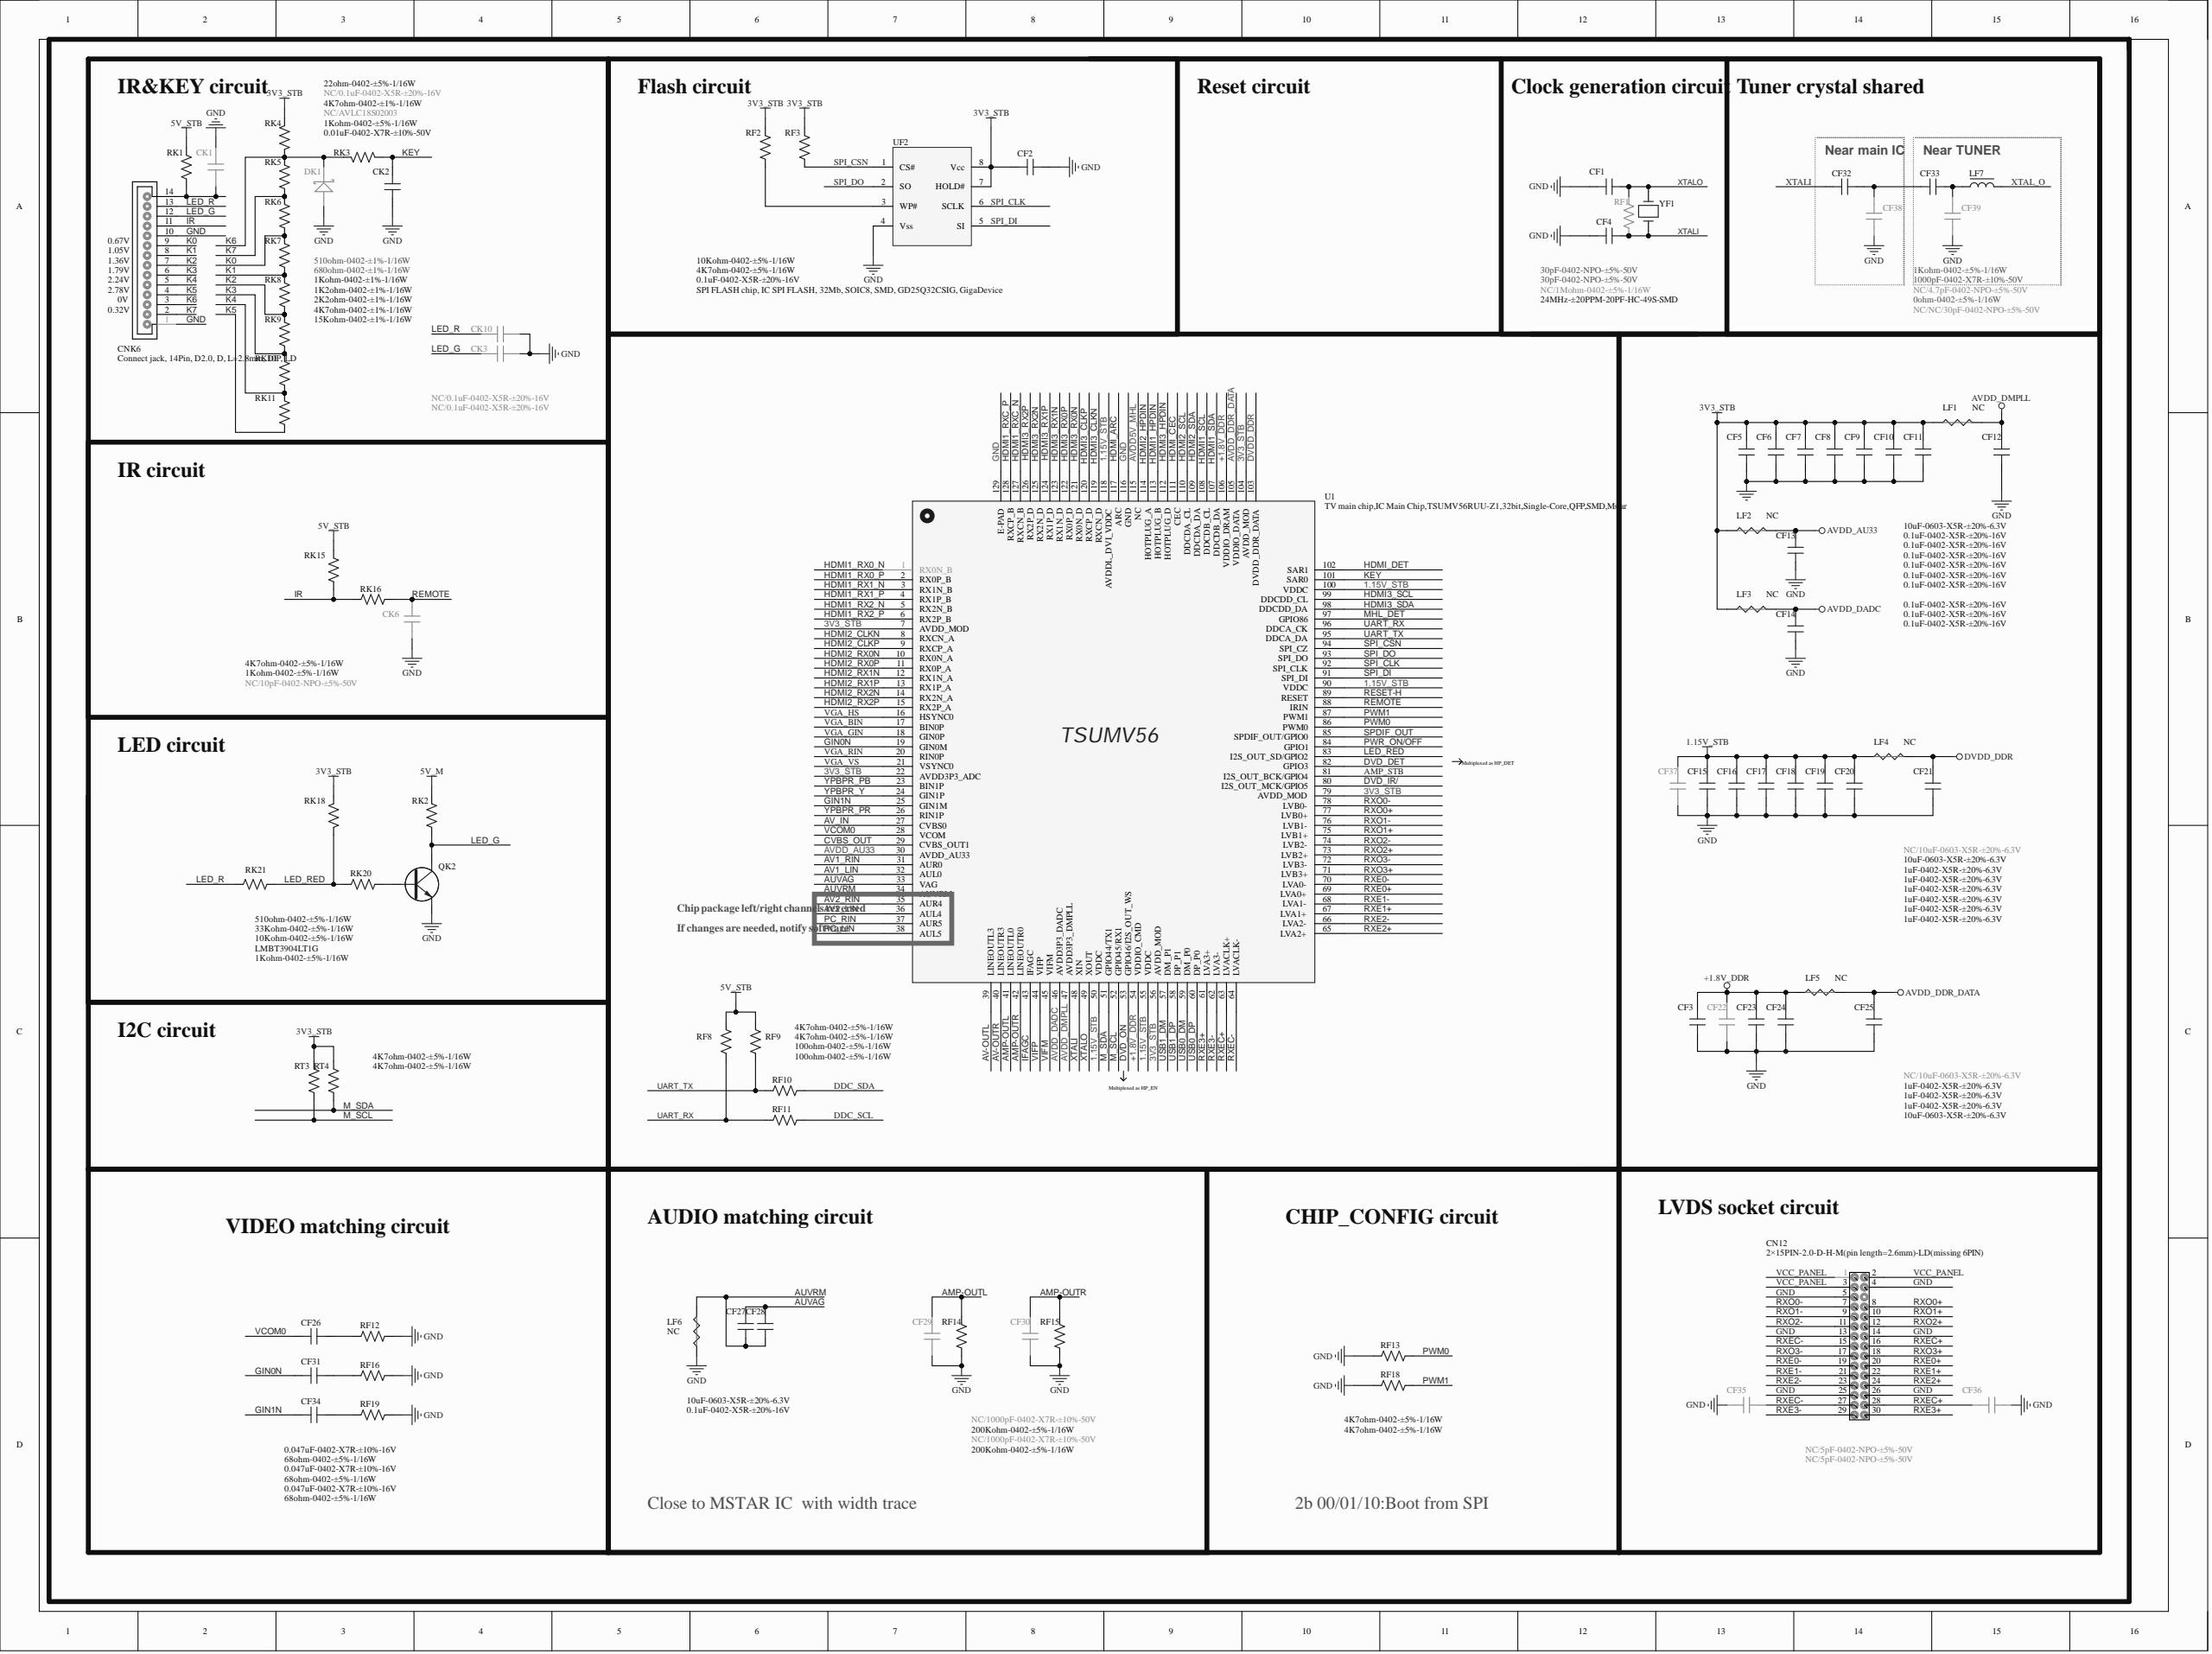Circuit board | Altium Designer | 709 parts | 378 nets | one sheet of the schematic
Parts on this sheet (reference | value | footprint):
CF1 | 30pF-0402-NPO-±5%-50V | C0402
CF2 | 0.1uF-0402-X5R-±20%-16V | C0402
CF3 | 10uF-0603-X5R-±20%-6.3V | C0603
CF4 | 30pF-0402-NPO-±5%-50V | C0402
CF5 | 10uF-0603-X5R-±20%-6.3V | C0603
CF6 | 0.1uF-0402-X5R-±20%-16V | C0402
CF7 | 0.1uF-0402-X5R-±20%-16V | C0402
CF8 | 0.1uF-0402-X5R-±20%-16V | C0402
CF9 | 0.1uF-0402-X5R-±20%-16V | C0402
CF10 | 0.1uF-0402-X5R-±20%-16V | C0402
CF11 | 0.1uF-0402-X5R-±20%-16V | C0402
CF12 | 0.1uF-0402-X5R-±20%-16V | C0402
CF13 | 0.1uF-0402-X5R-±20%-16V | C0402
CF14 | 0.1uF-0402-X5R-±20%-16V | C0402
CF15 | 10uF-0603-X5R-±20%-6.3V | C0603
CF16 | 1uF-0402-X5R-±20%-6.3V | C0402
CF17 | 1uF-0402-X5R-±20%-6.3V | C0402
CF18 | 1uF-0402-X5R-±20%-6.3V | C0402
CF19 | 1uF-0402-X5R-±20%-6.3V | C0402
CF20 | 1uF-0402-X5R-±20%-6.3V | C0402
CF21 | 1uF-0402-X5R-±20%-6.3V | C0402
CF22 | NC/10uF-0603-X5R-±20%-6.3V | C0603
CF23 | 1uF-0402-X5R-±20%-6.3V | C0402
CF24 | 1uF-0402-X5R-±20%-6.3V | C0402
CF25 | 1uF-0402-X5R-±20%-6.3V | C0402
CF26 | 0.047uF-0402-X7R-±10%-16V | C0402
CF27 | 0.1uF-0402-X5R-±20%-16V | C0402
CF28 | 10uF-0603-X5R-±20%-6.3V | C0603
CF29 | NC/1000pF-0402-X7R-±10%-50V | C0402
CF30 | NC/1000pF-0402-X7R-±10%-50V | C0402
CF31 | 0.047uF-0402-X7R-±10%-16V | C0402
CF32 | 1Kohm-0402-±5%-1/16W | C0402
CF33 | 1000pF-0402-X7R-±10%-50V | C0402
CF34 | 0.047uF-0402-X7R-±10%-16V | C0402
CF35 | NC/5pF-0402-NPO-±5%-50V | C0402
CF36 | NC/5pF-0402-NPO-±5%-50V | C0402
CF37 | NC/10uF-0603-X5R-±20%-6.3V | C0603
CF38 | NC/NC/30pF-0402-NPO-±5%-50V | C0402
CF39 | NC/4.7pF-0402-NPO-±5%-50V | C0402
CK1 | NC/0.1uF-0402-X5R-±20%-16V | C0402
CK2 | 0.01uF-0402-X7R-±10%-50V | C0402
CK3 | NC/0.1uF-0402-X5R-±20%-16V | C0402
CK6 | NC/10pF-0402-NPO-±5%-50V | C0402
CK10 | NC/0.1uF-0402-X5R-±20%-16V | C0402
CN12 | 2×15PIN-2.0-D-H-M(pin length=2.6mm)-LD(missing 6PIN) | SIP2*15/2.0D-2
CNK6 | Connect jack, 14Pin, D2.0, D, L=2.8mm, DIP, LD | SIP14/2.0D-1
DK1 | NC/AVLC18S02003 | DIODE-S0402
LF1 | NC | GND
LF2 | NC | GND
LF3 | NC | GND
LF4 | NC | GND
LF5 | NC | GND
LF6 | NC | GND
LF7 | 0ohm-0402-±5%-1/16W | L0402
QK2 | LMBT3904LT1G | SOT-23
RF1 | NC/1Mohm-0402-±5%-1/16W | R0402
RF2 | 10Kohm-0402-±5%-1/16W | R0402
RF3 | 4K7ohm-0402-±5%-1/16W | R0402
RF8 | 4K7ohm-0402-±5%-1/16W | R0402
RF9 | 4K7ohm-0402-±5%-1/16W | R0402
RF10 | 100ohm-0402-±5%-1/16W | R0402
RF11 | 100ohm-0402-±5%-1/16W | R0402
RF12 | 68ohm-0402-±5%-1/16W | R0402
RF13 | 4K7ohm-0402-±5%-1/16W | R0402
RF14 | 200Kohm-0402-±5%-1/16W | R0402
RF15 | 200Kohm-0402-±5%-1/16W | R0402
RF16 | 68ohm-0402-±5%-1/16W | R0402
RF18 | 4K7ohm-0402-±5%-1/16W | R0402
RF19 | 68ohm-0402-±5%-1/16W | R0402
RK1 | 22ohm-0402-±5%-1/16W | R0402
RK2 | 1Kohm-0402-±5%-1/16W | R0402
RK3 | 1Kohm-0402-±5%-1/16W | R0402
RK4 | 4K7ohm-0402-±1%-1/16W | R0402
RK5 | 510ohm-0402-±1%-1/16W | R0402
RK6 | 680ohm-0402-±1%-1/16W | R0402
RK7 | 1Kohm-0402-±1%-1/16W | R0402
RK8 | 1K2ohm-0402-±1%-1/16W | R0402
RK9 | 2K2ohm-0402-±1%-1/16W | R0402
RK10 | 4K7ohm-0402-±1%-1/16W | R0402
RK11 | 15Kohm-0402-±1%-1/16W | R0402
RK15 | 4K7ohm-0402-±5%-1/16W | R0402
RK16 | 1Kohm-0402-±5%-1/16W | R0402
RK18 | 33Kohm-0402-±5%-1/16W | R0402
RK20 | 10Kohm-0402-±5%-1/16W | R0402
RK21 | 510ohm-0402-±5%-1/16W | R0402
RT3 | 4K7ohm-0402-±5%-1/16W | R0402
RT4 | 4K7ohm-0402-±5%-1/16W | R0402
U1 | TV main chip,IC Main Chip,TSUMV56RUU-Z1,32bit,Single-Core,QFP,SMD,Mstar | QFP128/0.4-5
UF2 | SPI FLASH chip, IC SPI FLASH, 32Mb, SOIC8, SMD, GD25Q32CSIG, GigaDevice | SOIC8
YF1 | 24MHz-±20PPM-20PF-HC-49S-SMD | XTAL-S-1
Nets of these parts (net: part-pin ...):
YPBPR_Y: U1-24
YPBPR_PR: U1-26
YPBPR_PB: U1-23
XTALO: CF1-2 RF1-2 YF1-2 U1-49
XTALI: CF4-2 CF32-2 RF1-1 YF1-1 U1-48
XTAL_O: LF7-2
VIFP: U1-44
VIFM: U1-45
VGA_VS: U1-21
VGA_RIN: U1-20
VGA_HS: U1-16
VGA_GIN: U1-18
VGA_BIN: U1-17
VCOM0: CF26-1 U1-28
VCC_PANEL: CN12-1 CN12-2 CN12-3
USB1_DP: U1-58
USB1_DM: U1-57
USB0_DP: U1-60
USB0_DM: U1-59
UART_TX: RF9-1 RF10-1 U1-95
UART_RX: RF8-1 RF11-1 U1-96
SPI_DO: UF2-2 U1-93
SPI_DI: UF2-5 U1-91
SPI_CSN: RF3-1 UF2-1 U1-94
SPI_CLK: UF2-6 U1-92
SPDIF_OUT: U1-85
RXO3-: CN12-17 U1-72
RXO3+: CN12-18 U1-71
RXO2-: CN12-11 U1-74
RXO2+: CN12-12 U1-73
RXO1-: CN12-9 U1-76
RXO1+: CN12-10 U1-75
RXO0-: CN12-7 U1-78
RXO0+: CN12-8 U1-77
RXEC-: CF35-2 CN12-15 CN12-27 U1-64
RXEC+: CF36-1 CN12-16 CN12-28 U1-63
RXE3+: CN12-30 U1-61
RXE2-: CN12-23 U1-66
RXE2+: CN12-24 U1-65
RXE1-: CN12-21 U1-68
RXE1+: CN12-22 U1-67
RXE0-: CN12-19 U1-70
RXE0+: CN12-20 U1-69
REMOTE: CK6-2 RK16-1 U1-88
PWR_ON/OFF: U1-84
PWM1: RF18-1 U1-87
PWM0: RF13-1 U1-86
PC_RIN: U1-37
PC_LIN: U1-38
NetRF2_1: RF2-1 UF2-3
NetQK2_B: QK2-B RK20-1
NetCK1_2: CK1-2 CNK6-14 RK1-2
NetCF34_2: CF34-2 RF19-1
NetCF33_1: CF33-1 CF39-2 LF7-1
NetCF32_1: CF32-1 CF33-2 CF38-2
NetCF31_2: CF31-2 RF16-1
NetCF26_2: CF26-2 RF12-1
M_SDA: RT4-2 U1-51
M_SCL: RT3-2 U1-52
LED_RED: RK18-1 RK20-2 RK21-1 U1-83
LED_R: CK10-2 CNK6-13 RK21-2
LED_G: CK3-2 CNK6-12 QK2-C RK2-1
KEY: CK2-1 RK3-1 U1-101
K7: CNK6-2 RK5-2 RK6-2
K6: CNK6-3 DK1-K RK3-2 RK4-1 RK5-1
K5: CNK6-4 RK11-2
K4: CNK6-5 RK10-2 RK11-1
K3: CNK6-6 RK9-2 RK10-1
K2: CNK6-7 RK8-2 RK9-1
K1: CNK6-8 RK7-2 RK8-1
K0: CNK6-9 RK6-1 RK7-1
IR: CNK6-11 RK15-2 RK16-2
IFAGC: U1-43
HDMI_DET: U1-102
HDMI_CEC: U1-111
HDMI_ARC: U1-117
HDMI3_SDA: U1-98
HDMI3_SCL: U1-99
HDMI3_RX2P: U1-126
HDMI3_RX2N: U1-125
HDMI3_RX1P: U1-124
HDMI3_RX1N: U1-123
HDMI3_RX0P: U1-122
HDMI3_RX0N: U1-121
HDMI3_HPDIN: U1-112
HDMI3_CLKP: U1-120
HDMI3_CLKN: U1-119
HDMI1_SDA: U1-107
HDMI1_SCL: U1-108
HDMI1_RXC_P: U1-128
HDMI1_RXC_N: U1-127
HDMI1_RX2_P: U1-6
HDMI1_RX2_N: U1-5
HDMI1_RX1_P: U1-4
HDMI1_RX1_N: U1-3
HDMI1_RX0_P: U1-2
HDMI1_RX0_N: U1-1
HDMI1_HPDIN: U1-113
GND: CF1-1 CF2-1 CF3-2 CF4-1 CF5-2 CF6-1 CF7-1 CF8-1 CF9-1 CF10-1 CF11-1 CF12-1 CF13-1 CF14-1 CF15-2 CF16-1 CF17-1 CF18-1 CF19-1 CF20-1 CF21-1 CF22-2 CF23-1 CF24-1 CF25-1 CF29-2 CF30-2 CF35-1 CF36-2 CF37-2 CF38-1 CF39-1 CK1-1 CK2-2 CK3-1 CK6-1 CK10-1 CNK6-1 CNK6-10 DK1-A LF6-JP_2K QK2-E RF12-2 RF13-2 RF14-1 RF15-1 RF16-2 RF18-2 RF19-2 UF2-4 CN12-4 CN12-5 CN12-13 CN12-14 CN12-25 CN12-26 U1-116 U1-129
GIN1N: CF34-1 U1-25
GIN0N: CF31-1 U1-19
DVDD_DDR: CF21-2 LF4-JP_1K U1-103
DDC_SDA: RF10-2
DDC_SCL: RF11-2
CVBS_OUT: U1-29
AVDD_DMPLL: CF12-2 LF1-JP_1K U1-47
AVDD_DDR_DATA: CF25-2 LF5-JP_1K U1-105
AVDD_DADC: CF14-2 LF3-JP_1K U1-46
AVDD_AU33: CF13-2 LF2-JP_1K U1-30
AV_IN: U1-27
AV-OUTR: U1-40
AV-OUTL: U1-39
AV2_RIN: U1-35
AV2_LIN: U1-36
AV1_RIN: U1-31
AV1_LIN: U1-32
AUVRM: CF27-1 CF28-2 LF6-JP_1K U1-34
AUVAG: CF27-2 CF28-1 U1-33
AMP_STB: U1-81
AMP-OUTR: CF30-1 RF15-2 U1-42
AMP-OUTL: CF29-1 RF14-2 U1-41
+1.8V_DDR: CF3-1 CF22-1 CF23-2 CF24-2 LF5-JP_2K U1-54 U1-106
5V_STB: RF8-2 RF9-2 RK1-1 RK15-1
5V_M: RK2-2
3V3_STB: CF2-2 CF5-1 CF6-2 CF7-2 CF8-2 CF9-2 CF10-2 CF11-2 LF1-JP_2K LF2-JP_2K LF3-JP_2K RF2-2 RF3-2 RK4-2 RK18-2 RT3-1 RT4-1 UF2-7 UF2-8 U1-7 U1-22 U1-56 U1-79 U1-104
1.15V_STB: CF15-1 CF16-2 CF17-2 CF18-2 CF19-2 CF20-2 CF37-1 LF4-JP_2K U1-50 U1-55 U1-90 U1-100 U1-118